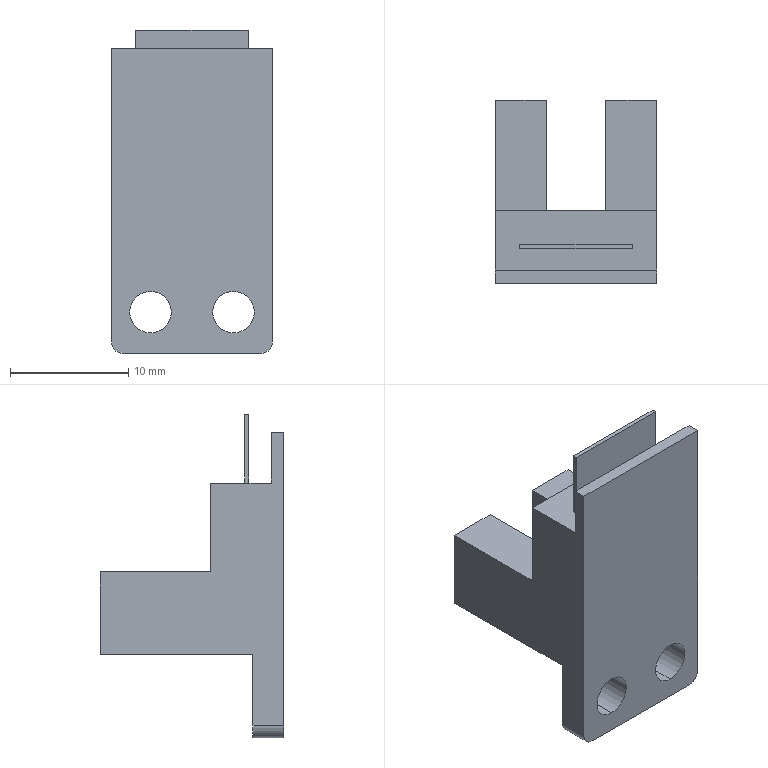Part | STEP file | xgSENSOR(EE-SX674) | 1 solid | 27 faces | box 13.6 x 15.5 x 27.3 mm | volume 2060 mm3 | plane 21 | cylinder 6 | commonest cylinder face diameters 3.5 x4 2 x2